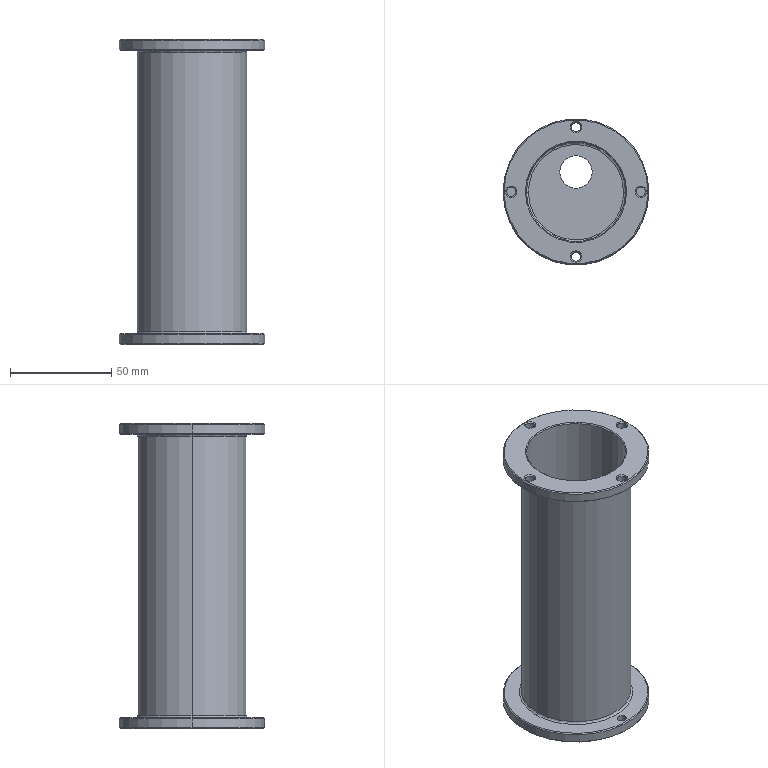Part | STEP file | Fix sleeve | 1 solid | 215 faces | box 72 x 72 x 150.6 mm | volume 87626 mm3 | spline 89 | plane 52 | cylinder 50 | cone 24 | commonest cylinder face diameters 53.98 x22 4.6 x8 54 x8 4.5 x4 72 x4 16 x2